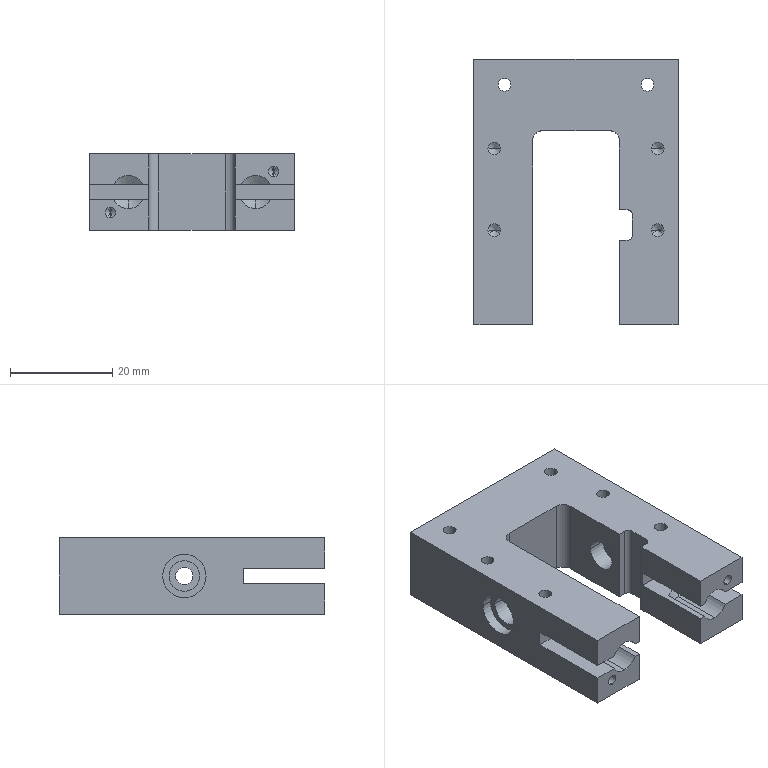Part | NX | features BREP 1 | 1 solid | 79 faces | box 40 x 52 x 15 mm | volume 18952 mm3 | cylinder 36 | plane 25 | cone 18 | commonest cylinder face diameters 2.5 x12 6 x6 6.5 x6 2.05 x4 2 x2 3.4 x2